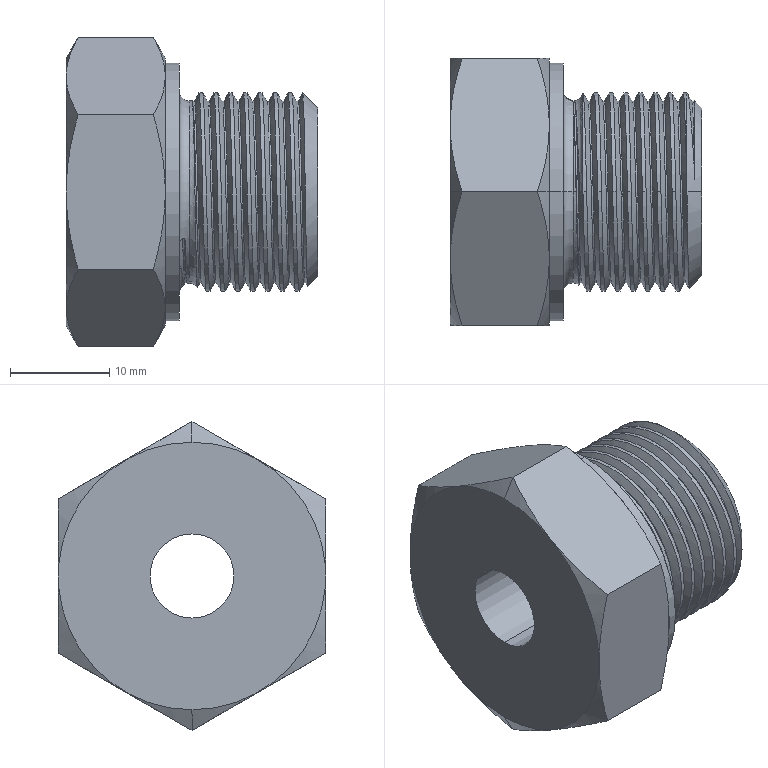Part | SolidWorks | features ICE 3, Chamfer 1, Revolution 1, SweepThread 1 | 1 solid | 47 faces | box 25.4 x 27.003 x 31.18 mm | volume 9595 mm3 | cylinder 19 | plane 11 | torus 7 | cone 6 | spline 4 | commonest cylinder face diameters 20 x15 8.5 x2 26 x2